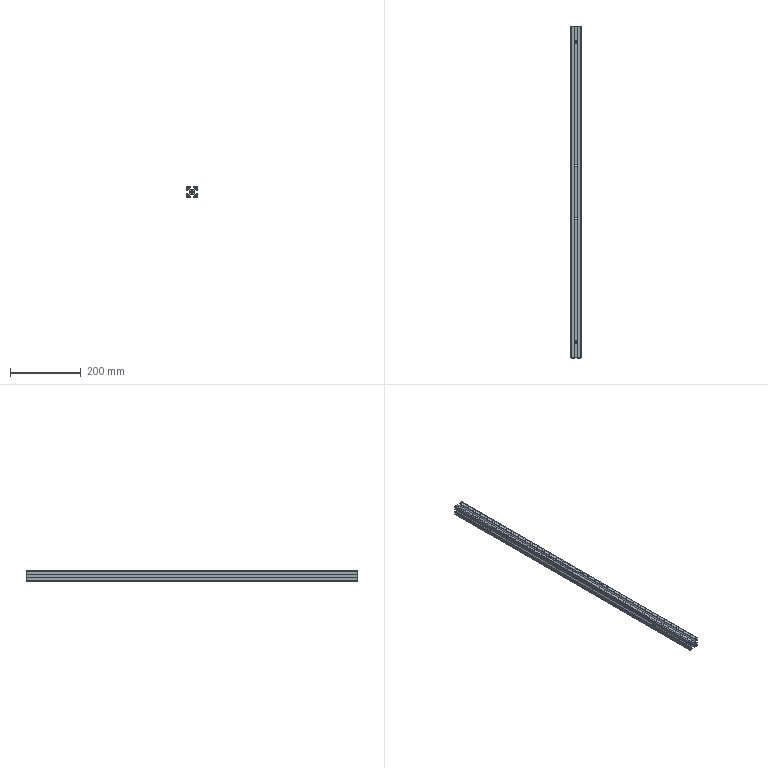Part | SolidWorks | features Extrusion 1, HoleWzd 1 | 1 solid | 108 faces | box 30 x 940 x 30 mm | volume 311608 mm3 | cylinder 54 | plane 54 | commonest cylinder face diameters 11 x24 6.6 x16 4.2 x8 4 x4 6.8 x2